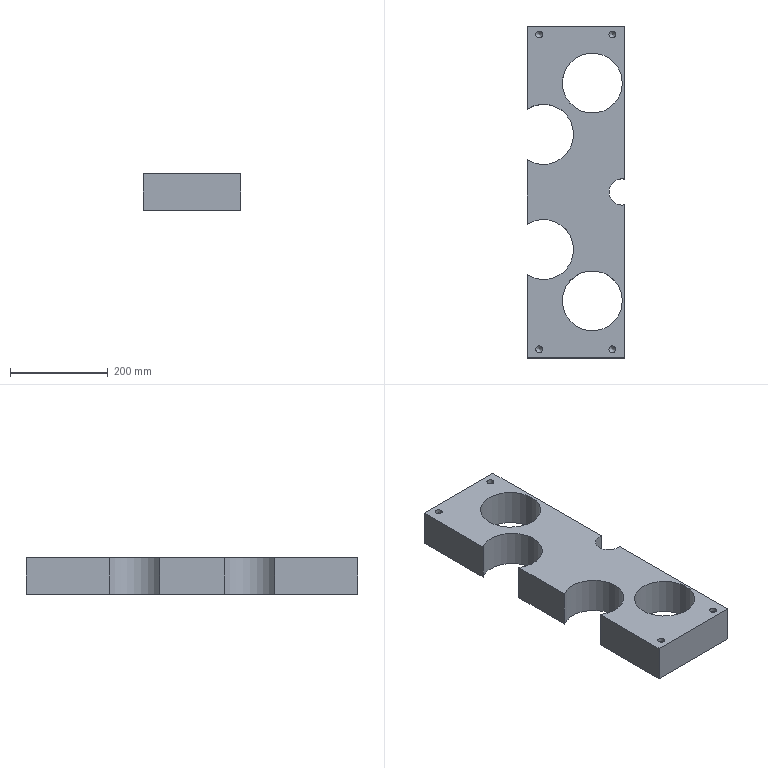Part | NX | features 3 2 | 1 solid | 30 faces | box 199 x 680 x 75.5 mm | volume 6823657 mm3 | cylinder 13 | plane 9 | cone 8 | commonest cylinder face diameters 14.1 x8 123 x4 54 x1
STEP:
#1=CARTESIAN_POINT('',(1737.05,322.5,256.5));
#2=VERTEX_POINT('',#1);
#3=CARTESIAN_POINT('',(1730.,322.5,256.5));
#4=DIRECTION('',(0.,0.,-1.));
#5=DIRECTION('',(1.,0.,0.));
#6=AXIS2_PLACEMENT_3D('',#3,#4,#5);
#7=CIRCLE('',#6,7.05);
#8=EDGE_CURVE('',#2,#2,#7,.T.);
#9=ORIENTED_EDGE('',*,*,#8,.T.);
#10=EDGE_LOOP('',(#9));
#11=FACE_BOUND('',#10,.T.);
#12=CARTESIAN_POINT('',(1587.05,-322.5,256.5));
#13=VERTEX_POINT('',#12);
#14=CARTESIAN_POINT('',(1580.,-322.5,256.5));
#15=DIRECTION('',(0.,0.,-1.));
#16=DIRECTION('',(1.,0.,0.));
#17=AXIS2_PLACEMENT_3D('',#14,#15,#16);
#18=CIRCLE('',#17,7.05);
#19=EDGE_CURVE('',#13,#13,#18,.T.);
#20=ORIENTED_EDGE('',*,*,#19,.T.);
#21=EDGE_LOOP('',(#20));
#22=FACE_BOUND('',#21,.T.);
#23=CARTESIAN_POINT('',(1750.5,-223.,256.5));
#24=VERTEX_POINT('',#23);
#25=CARTESIAN_POINT('',(1689.,-223.,256.5));
#26=DIRECTION('',(0.,0.,1.));
#27=DIRECTION('',(1.,0.,0.));
#28=AXIS2_PLACEMENT_3D('',#25,#26,#27);
#29=CIRCLE('',#28,61.5);
#30=EDGE_CURVE('',#24,#24,#29,.T.);
#31=ORIENTED_EDGE('',*,*,#30,.F.);
#32=EDGE_LOOP('',(#31));
#33=FACE_BOUND('',#32,.T.);
#34=CARTESIAN_POINT('',(1750.5,223.,256.5));
#35=VERTEX_POINT('',#34);
#36=CARTESIAN_POINT('',(1689.,223.,256.5));
#37=DIRECTION('',(0.,0.,-1.));
#38=DIRECTION('',(1.,0.,0.));
#39=AXIS2_PLACEMENT_3D('',#36,#37,#38);
#40=CIRCLE('',#39,61.5);
#41=EDGE_CURVE('',#35,#35,#40,.T.);
#42=ORIENTED_EDGE('',*,*,#41,.T.);
#43=EDGE_LOOP('',(#42));
#44=FACE_BOUND('',#43,.T.);
#45=CARTESIAN_POINT('',(1755.,-26.533,256.5));
#46=VERTEX_POINT('',#45);
#47=CARTESIAN_POINT('',(1755.,-340.,256.5));
#48=VERTEX_POINT('',#47);
#49=CARTESIAN_POINT('',(1755.,193.,256.5));
#50=DIRECTION('',(0.,-1.,0.));
#51=VECTOR('',#50,1000.);
#52=LINE('',#49,#51);
#53=EDGE_CURVE('',#46,#48,#52,.T.);
#54=ORIENTED_EDGE('',*,*,#53,.F.);
#55=CARTESIAN_POINT('',(1755.,26.533,256.5));
#56=VERTEX_POINT('',#55);
#57=CARTESIAN_POINT('',(1750.,0.,256.5));
#58=DIRECTION('',(0.,0.,-1.));
#59=DIRECTION('',(1.,0.,0.));
#60=AXIS2_PLACEMENT_3D('',#57,#58,#59);
#61=CIRCLE('',#60,27.);
#62=EDGE_CURVE('',#46,#56,#61,.T.);
#63=ORIENTED_EDGE('',*,*,#62,.T.);
#64=CARTESIAN_POINT('',(1755.,340.,256.5));
#65=VERTEX_POINT('',#64);
#66=CARTESIAN_POINT('',(1755.,193.,256.5));
#67=DIRECTION('',(0.,-1.,0.));
#68=VECTOR('',#67,1000.);
#69=LINE('',#66,#68);
#70=EDGE_CURVE('',#65,#56,#69,.T.);
#71=ORIENTED_EDGE('',*,*,#70,.F.);
#72=CARTESIAN_POINT('',(1556.,340.,256.5));
#73=VERTEX_POINT('',#72);
#74=CARTESIAN_POINT('',(1447.,340.,256.5));
#75=DIRECTION('',(-1.,0.,0.));
#76=VECTOR('',#75,1000.);
#77=LINE('',#74,#76);
#78=EDGE_CURVE('',#65,#73,#77,.T.);
#79=ORIENTED_EDGE('',*,*,#78,.T.);
#80=CARTESIAN_POINT('',(1556.,169.897,256.5));
#81=VERTEX_POINT('',#80);
#82=CARTESIAN_POINT('',(1556.,-1700.,256.5));
#83=DIRECTION('',(0.,1.,0.));
#84=VECTOR('',#83,1000.);
#85=LINE('',#82,#84);
#86=EDGE_CURVE('',#81,#73,#85,.T.);
#87=ORIENTED_EDGE('',*,*,#86,.F.);
#88=CARTESIAN_POINT('',(1556.,66.103,256.5));
#89=VERTEX_POINT('',#88);
#90=CARTESIAN_POINT('',(1589.,118.,256.5));
#91=DIRECTION('',(0.,0.,1.));
#92=DIRECTION('',(1.,0.,0.));
#93=AXIS2_PLACEMENT_3D('',#90,#91,#92);
#94=CIRCLE('',#93,61.5);
#95=EDGE_CURVE('',#89,#81,#94,.T.);
#96=ORIENTED_EDGE('',*,*,#95,.F.);
#97=CARTESIAN_POINT('',(1556.,-66.103,256.5));
#98=VERTEX_POINT('',#97);
#99=CARTESIAN_POINT('',(1556.,-1700.,256.5));
#100=DIRECTION('',(0.,1.,0.));
#101=VECTOR('',#100,1000.);
#102=LINE('',#99,#101);
#103=EDGE_CURVE('',#98,#89,#102,.T.);
#104=ORIENTED_EDGE('',*,*,#103,.F.);
#105=CARTESIAN_POINT('',(1556.,-169.897,256.5));
#106=VERTEX_POINT('',#105);
#107=CARTESIAN_POINT('',(1589.,-118.,256.5));
#108=DIRECTION('',(0.,0.,-1.));
#109=DIRECTION('',(1.,0.,0.));
#110=AXIS2_PLACEMENT_3D('',#107,#108,#109);
#111=CIRCLE('',#110,61.5);
#112=EDGE_CURVE('',#98,#106,#111,.T.);
#113=ORIENTED_EDGE('',*,*,#112,.T.);
#114=CARTESIAN_POINT('',(1556.,-340.,256.5));
#115=VERTEX_POINT('',#114);
#116=CARTESIAN_POINT('',(1556.,-1700.,256.5));
#117=DIRECTION('',(0.,1.,0.));
#118=VECTOR('',#117,1000.);
#119=LINE('',#116,#118);
#120=EDGE_CURVE('',#115,#106,#119,.T.);
#121=ORIENTED_EDGE('',*,*,#120,.F.);
#122=CARTESIAN_POINT('',(1640.,-340.,256.5));
#123=DIRECTION('',(1.,0.,0.));
#124=VECTOR('',#123,1000.);
#125=LINE('',#122,#124);
#126=EDGE_CURVE('',#115,#48,#125,.T.);
#127=ORIENTED_EDGE('',*,*,#126,.T.);
#128=EDGE_LOOP('',(#54,#63,#71,#79,#87,#96,#104,#113,#121,#127));
#129=FACE_BOUND('',#128,.T.);
#130=CARTESIAN_POINT('',(1587.05,322.5,256.5));
#131=VERTEX_POINT('',#130);
#132=CARTESIAN_POINT('',(1580.,322.5,256.5));
#133=DIRECTION('',(0.,0.,-1.));
#134=DIRECTION('',(1.,0.,0.));
#135=AXIS2_PLACEMENT_3D('',#132,#133,#134);
#136=CIRCLE('',#135,7.05);
#137=EDGE_CURVE('',#131,#131,#136,.T.);
#138=ORIENTED_EDGE('',*,*,#137,.T.);
#139=EDGE_LOOP('',(#138));
#140=FACE_BOUND('',#139,.T.);
#141=CARTESIAN_POINT('',(1737.05,-322.5,256.5));
#142=VERTEX_POINT('',#141);
#143=CARTESIAN_POINT('',(1730.,-322.5,256.5));
#144=DIRECTION('',(0.,0.,-1.));
#145=DIRECTION('',(1.,0.,0.));
#146=AXIS2_PLACEMENT_3D('',#143,#144,#145);
#147=CIRCLE('',#146,7.05);
#148=EDGE_CURVE('',#142,#142,#147,.T.);
#149=ORIENTED_EDGE('',*,*,#148,.T.);
#150=EDGE_LOOP('',(#149));
#151=FACE_BOUND('',#150,.T.);
#152=CARTESIAN_POINT('',(1640.,-1700.,256.5));
#153=DIRECTION('',(0.,0.,1.));
#154=DIRECTION('',(0.,1.,0.));
#155=AXIS2_PLACEMENT_3D('',#152,#153,#154);
#156=PLANE('',#155);
#157=ADVANCED_FACE('',(#11,#22,#33,#44,#129,#140,#151),#156,.T.);
#158=CARTESIAN_POINT('',(1738.05,-127.5,181.));
#159=VERTEX_POINT('',#158);
#160=CARTESIAN_POINT('',(1731.,-127.5,181.));
#161=DIRECTION('',(0.,0.,1.));
#162=DIRECTION('',(1.,0.,0.));
#163=AXIS2_PLACEMENT_3D('',#160,#161,#162);
#164=CIRCLE('',#163,7.05);
#165=EDGE_CURVE('',#159,#159,#164,.T.);
#166=ORIENTED_EDGE('',*,*,#165,.T.);
#167=EDGE_LOOP('',(#166));
#168=FACE_BOUND('',#167,.T.);
#169=CARTESIAN_POINT('',(1738.05,127.5,181.));
#170=VERTEX_POINT('',#169);
#171=CARTESIAN_POINT('',(1731.,127.5,181.));
#172=DIRECTION('',(0.,0.,1.));
#173=DIRECTION('',(1.,0.,0.));
#174=AXIS2_PLACEMENT_3D('',#171,#172,#173);
#175=CIRCLE('',#174,7.05);
#176=EDGE_CURVE('',#170,#170,#175,.T.);
#177=ORIENTED_EDGE('',*,*,#176,.T.);
#178=EDGE_LOOP('',(#177));
#179=FACE_BOUND('',#178,.T.);
#180=CARTESIAN_POINT('',(1627.5,-223.,181.));
#181=VERTEX_POINT('',#180);
#182=CARTESIAN_POINT('',(1689.,-223.,181.));
#183=DIRECTION('',(0.,0.,-1.));
#184=DIRECTION('',(-1.,0.,0.));
#185=AXIS2_PLACEMENT_3D('',#182,#183,#184);
#186=CIRCLE('',#185,61.5);
#187=EDGE_CURVE('',#181,#181,#186,.T.);
#188=ORIENTED_EDGE('',*,*,#187,.F.);
#189=EDGE_LOOP('',(#188));
#190=FACE_BOUND('',#189,.T.);
#191=CARTESIAN_POINT('',(1627.5,223.,181.));
#192=VERTEX_POINT('',#191);
#193=CARTESIAN_POINT('',(1689.,223.,181.));
#194=DIRECTION('',(0.,0.,1.));
#195=DIRECTION('',(-1.,0.,0.));
#196=AXIS2_PLACEMENT_3D('',#193,#194,#195);
#197=CIRCLE('',#196,61.5);
#198=EDGE_CURVE('',#192,#192,#197,.T.);
#199=ORIENTED_EDGE('',*,*,#198,.T.);
#200=EDGE_LOOP('',(#199));
#201=FACE_BOUND('',#200,.T.);
#202=CARTESIAN_POINT('',(1755.,26.533,181.));
#203=VERTEX_POINT('',#202);
#204=CARTESIAN_POINT('',(1755.,340.,181.));
#205=VERTEX_POINT('',#204);
#206=CARTESIAN_POINT('',(1755.,193.,181.));
#207=DIRECTION('',(0.,1.,0.));
#208=VECTOR('',#207,1000.);
#209=LINE('',#206,#208);
#210=EDGE_CURVE('',#203,#205,#209,.T.);
#211=ORIENTED_EDGE('',*,*,#210,.F.);
#212=CARTESIAN_POINT('',(1755.,-26.533,181.));
#213=VERTEX_POINT('',#212);
#214=CARTESIAN_POINT('',(1750.,0.,181.));
#215=DIRECTION('',(0.,0.,1.));
#216=DIRECTION('',(-1.,0.,0.));
#217=AXIS2_PLACEMENT_3D('',#214,#215,#216);
#218=CIRCLE('',#217,27.);
#219=EDGE_CURVE('',#203,#213,#218,.T.);
#220=ORIENTED_EDGE('',*,*,#219,.T.);
#221=CARTESIAN_POINT('',(1755.,-340.,181.));
#222=VERTEX_POINT('',#221);
#223=CARTESIAN_POINT('',(1755.,193.,181.));
#224=DIRECTION('',(0.,1.,0.));
#225=VECTOR('',#224,1000.);
#226=LINE('',#223,#225);
#227=EDGE_CURVE('',#222,#213,#226,.T.);
#228=ORIENTED_EDGE('',*,*,#227,.F.);
#229=CARTESIAN_POINT('',(1556.,-340.,181.));
#230=VERTEX_POINT('',#229);
#231=CARTESIAN_POINT('',(1447.,-340.,181.));
#232=DIRECTION('',(-1.,0.,0.));
#233=VECTOR('',#232,1000.);
#234=LINE('',#231,#233);
#235=EDGE_CURVE('',#222,#230,#234,.T.);
#236=ORIENTED_EDGE('',*,*,#235,.T.);
#237=CARTESIAN_POINT('',(1556.,-169.897,181.));
#238=VERTEX_POINT('',#237);
#239=CARTESIAN_POINT('',(1556.,-930.,181.));
#240=DIRECTION('',(0.,-1.,0.));
#241=VECTOR('',#240,1000.);
#242=LINE('',#239,#241);
#243=EDGE_CURVE('',#238,#230,#242,.T.);
#244=ORIENTED_EDGE('',*,*,#243,.F.);
#245=CARTESIAN_POINT('',(1556.,-66.103,181.));
#246=VERTEX_POINT('',#245);
#247=CARTESIAN_POINT('',(1589.,-118.,181.));
#248=DIRECTION('',(0.,0.,-1.));
#249=DIRECTION('',(-1.,0.,0.));
#250=AXIS2_PLACEMENT_3D('',#247,#248,#249);
#251=CIRCLE('',#250,61.5);
#252=EDGE_CURVE('',#246,#238,#251,.T.);
#253=ORIENTED_EDGE('',*,*,#252,.F.);
#254=CARTESIAN_POINT('',(1556.,66.103,181.));
#255=VERTEX_POINT('',#254);
#256=CARTESIAN_POINT('',(1556.,-930.,181.));
#257=DIRECTION('',(0.,-1.,0.));
#258=VECTOR('',#257,1000.);
#259=LINE('',#256,#258);
#260=EDGE_CURVE('',#255,#246,#259,.T.);
#261=ORIENTED_EDGE('',*,*,#260,.F.);
#262=CARTESIAN_POINT('',(1556.,169.897,181.));
#263=VERTEX_POINT('',#262);
#264=CARTESIAN_POINT('',(1589.,118.,181.));
#265=DIRECTION('',(0.,0.,1.));
#266=DIRECTION('',(-1.,0.,0.));
#267=AXIS2_PLACEMENT_3D('',#264,#265,#266);
#268=CIRCLE('',#267,61.5);
#269=EDGE_CURVE('',#255,#263,#268,.T.);
#270=ORIENTED_EDGE('',*,*,#269,.T.);
#271=CARTESIAN_POINT('',(1556.,340.,181.));
#272=VERTEX_POINT('',#271);
#273=CARTESIAN_POINT('',(1556.,-930.,181.));
#274=DIRECTION('',(0.,-1.,0.));
#275=VECTOR('',#274,1000.);
#276=LINE('',#273,#275);
#277=EDGE_CURVE('',#272,#263,#276,.T.);
#278=ORIENTED_EDGE('',*,*,#277,.F.);
#279=CARTESIAN_POINT('',(1447.,340.,181.));
#280=DIRECTION('',(1.,0.,0.));
#281=VECTOR('',#280,1000.);
#282=LINE('',#279,#281);
#283=EDGE_CURVE('',#272,#205,#282,.T.);
#284=ORIENTED_EDGE('',*,*,#283,.T.);
#285=EDGE_LOOP('',(#211,#220,#228,#236,#244,#253,#261,#270,#278,#284));
#286=FACE_BOUND('',#285,.T.);
#287=CARTESIAN_POINT('',(1587.05,-322.5,181.));
#288=VERTEX_POINT('',#287);
#289=CARTESIAN_POINT('',(1580.,-322.5,181.));
#290=DIRECTION('',(0.,0.,1.));
#291=DIRECTION('',(1.,0.,0.));
#292=AXIS2_PLACEMENT_3D('',#289,#290,#291);
#293=CIRCLE('',#292,7.05);
#294=EDGE_CURVE('',#288,#288,#293,.T.);
#295=ORIENTED_EDGE('',*,*,#294,.T.);
#296=EDGE_LOOP('',(#295));
#297=FACE_BOUND('',#296,.T.);
#298=CARTESIAN_POINT('',(1587.05,322.5,181.));
#299=VERTEX_POINT('',#298);
#300=CARTESIAN_POINT('',(1580.,322.5,181.));
#301=DIRECTION('',(0.,0.,1.));
#302=DIRECTION('',(1.,0.,0.));
#303=AXIS2_PLACEMENT_3D('',#300,#301,#302);
#304=CIRCLE('',#303,7.05);
#305=EDGE_CURVE('',#299,#299,#304,.T.);
#306=ORIENTED_EDGE('',*,*,#305,.T.);
#307=EDGE_LOOP('',(#306));
#308=FACE_BOUND('',#307,.T.);
#309=CARTESIAN_POINT('',(1447.,-930.,181.));
#310=DIRECTION('',(0.,0.,-1.));
#311=DIRECTION('',(0.,1.,0.));
#312=AXIS2_PLACEMENT_3D('',#309,#310,#311);
#313=PLANE('',#312);
#314=ADVANCED_FACE('',(#168,#179,#190,#201,#286,#297,#308),#313,.T.);
#315=ORIENTED_EDGE('',*,*,#70,.T.);
#316=CARTESIAN_POINT('',(1755.,26.533,-181.));
#317=DIRECTION('',(0.,0.,-1.));
#318=VECTOR('',#317,1000.);
#319=LINE('',#316,#318);
#320=EDGE_CURVE('',#56,#203,#319,.T.);
#321=ORIENTED_EDGE('',*,*,#320,.T.);
#322=ORIENTED_EDGE('',*,*,#210,.T.);
#323=CARTESIAN_POINT('',(1755.,340.,-1.5));
#324=DIRECTION('',(0.,0.,1.));
#325=VECTOR('',#324,1000.);
#326=LINE('',#323,#325);
#327=EDGE_CURVE('',#205,#65,#326,.T.);
#328=ORIENTED_EDGE('',*,*,#327,.T.);
#329=EDGE_LOOP('',(#315,#321,#322,#328));
#330=FACE_BOUND('',#329,.T.);
#331=CARTESIAN_POINT('',(1755.,193.,-1.5));
#332=DIRECTION('',(1.,0.,0.));
#333=DIRECTION('',(0.,0.,1.));
#334=AXIS2_PLACEMENT_3D('',#331,#332,#333);
#335=PLANE('',#334);
#336=ADVANCED_FACE('',(#330),#335,.T.);
#337=ORIENTED_EDGE('',*,*,#227,.T.);
#338=CARTESIAN_POINT('',(1755.,-26.533,-181.));
#339=DIRECTION('',(0.,0.,1.));
#340=VECTOR('',#339,1000.);
#341=LINE('',#338,#340);
#342=EDGE_CURVE('',#213,#46,#341,.T.);
#343=ORIENTED_EDGE('',*,*,#342,.T.);
#344=ORIENTED_EDGE('',*,*,#53,.T.);
#345=CARTESIAN_POINT('',(1755.,-340.,-1.5));
#346=DIRECTION('',(0.,0.,-1.));
#347=VECTOR('',#346,1000.);
#348=LINE('',#345,#347);
#349=EDGE_CURVE('',#48,#222,#348,.T.);
#350=ORIENTED_EDGE('',*,*,#349,.T.);
#351=EDGE_LOOP('',(#337,#343,#344,#350));
#352=FACE_BOUND('',#351,.T.);
#353=CARTESIAN_POINT('',(1755.,193.,-1.5));
#354=DIRECTION('',(1.,0.,0.));
#355=DIRECTION('',(0.,0.,1.));
#356=AXIS2_PLACEMENT_3D('',#353,#354,#355);
#357=PLANE('',#356);
#358=ADVANCED_FACE('',(#352),#357,.T.);
#359=ORIENTED_EDGE('',*,*,#103,.T.);
#360=CARTESIAN_POINT('',(1556.,66.103,-181.));
#361=DIRECTION('',(0.,0.,-1.));
#362=VECTOR('',#361,1000.);
#363=LINE('',#360,#362);
#364=EDGE_CURVE('',#89,#255,#363,.T.);
#365=ORIENTED_EDGE('',*,*,#364,.T.);
#366=ORIENTED_EDGE('',*,*,#260,.T.);
#367=CARTESIAN_POINT('',(1556.,-66.103,-181.));
#368=DIRECTION('',(0.,0.,1.));
#369=VECTOR('',#368,1000.);
#370=LINE('',#367,#369);
#371=EDGE_CURVE('',#246,#98,#370,.T.);
#372=ORIENTED_EDGE('',*,*,#371,.T.);
#373=EDGE_LOOP('',(#359,#365,#366,#372));
#374=FACE_BOUND('',#373,.T.);
#375=CARTESIAN_POINT('',(1556.,315.,218.75));
#376=DIRECTION('',(-1.,0.,0.));
#377=DIRECTION('',(0.,0.,-1.));
#378=AXIS2_PLACEMENT_3D('',#375,#376,#377);
#379=PLANE('',#378);
#380=ADVANCED_FACE('',(#374),#379,.T.);
#381=ORIENTED_EDGE('',*,*,#277,.T.);
#382=CARTESIAN_POINT('',(1556.,169.897,-181.));
#383=DIRECTION('',(0.,0.,1.));
#384=VECTOR('',#383,1000.);
#385=LINE('',#382,#384);
#386=EDGE_CURVE('',#263,#81,#385,.T.);
#387=ORIENTED_EDGE('',*,*,#386,.T.);
#388=ORIENTED_EDGE('',*,*,#86,.T.);
#389=CARTESIAN_POINT('',(1556.,340.,-1.5));
#390=DIRECTION('',(0.,0.,-1.));
#391=VECTOR('',#390,1000.);
#392=LINE('',#389,#391);
#393=EDGE_CURVE('',#73,#272,#392,.T.);
#394=ORIENTED_EDGE('',*,*,#393,.T.);
#395=EDGE_LOOP('',(#381,#387,#388,#394));
#396=FACE_BOUND('',#395,.T.);
#397=CARTESIAN_POINT('',(1556.,315.,218.75));
#398=DIRECTION('',(-1.,0.,0.));
#399=DIRECTION('',(0.,0.,-1.));
#400=AXIS2_PLACEMENT_3D('',#397,#398,#399);
#401=PLANE('',#400);
#402=ADVANCED_FACE('',(#396),#401,.T.);
#403=ORIENTED_EDGE('',*,*,#120,.T.);
#404=CARTESIAN_POINT('',(1556.,-169.897,-181.));
#405=DIRECTION('',(0.,0.,-1.));
#406=VECTOR('',#405,1000.);
#407=LINE('',#404,#406);
#408=EDGE_CURVE('',#106,#238,#407,.T.);
#409=ORIENTED_EDGE('',*,*,#408,.T.);
#410=ORIENTED_EDGE('',*,*,#243,.T.);
#411=CARTESIAN_POINT('',(1556.,-340.,218.75));
#412=DIRECTION('',(0.,0.,1.));
#413=VECTOR('',#412,1000.);
#414=LINE('',#411,#413);
#415=EDGE_CURVE('',#230,#115,#414,.T.);
#416=ORIENTED_EDGE('',*,*,#415,.T.);
#417=EDGE_LOOP('',(#403,#409,#410,#416));
#418=FACE_BOUND('',#417,.T.);
#419=CARTESIAN_POINT('',(1556.,315.,218.75));
#420=DIRECTION('',(-1.,0.,0.));
#421=DIRECTION('',(0.,0.,-1.));
#422=AXIS2_PLACEMENT_3D('',#419,#420,#421);
#423=PLANE('',#422);
#424=ADVANCED_FACE('',(#418),#423,.T.);
#425=ORIENTED_EDGE('',*,*,#283,.F.);
#426=ORIENTED_EDGE('',*,*,#393,.F.);
#427=ORIENTED_EDGE('',*,*,#78,.F.);
#428=ORIENTED_EDGE('',*,*,#327,.F.);
#429=EDGE_LOOP('',(#425,#426,#427,#428));
#430=FACE_BOUND('',#429,.T.);
#431=CARTESIAN_POINT('',(1447.,340.,-1.5));
#432=DIRECTION('',(0.,1.,0.));
#433=DIRECTION('',(0.,0.,-1.));
#434=AXIS2_PLACEMENT_3D('',#431,#432,#433);
#435=PLANE('',#434);
#436=ADVANCED_FACE('',(#430),#435,.T.);
#437=ORIENTED_EDGE('',*,*,#126,.F.);
#438=ORIENTED_EDGE('',*,*,#415,.F.);
#439=ORIENTED_EDGE('',*,*,#235,.F.);
#440=ORIENTED_EDGE('',*,*,#349,.F.);
#441=EDGE_LOOP('',(#437,#438,#439,#440));
#442=FACE_BOUND('',#441,.T.);
#443=CARTESIAN_POINT('',(1447.,-340.,-1.5));
#444=DIRECTION('',(0.,-1.,0.));
#445=DIRECTION('',(0.,0.,-1.));
#446=AXIS2_PLACEMENT_3D('',#443,#444,#445);
#447=PLANE('',#446);
#448=ADVANCED_FACE('',(#442),#447,.T.);
#449=ORIENTED_EDGE('',*,*,#30,.T.);
#450=EDGE_LOOP('',(#449));
#451=FACE_BOUND('',#450,.T.);
#452=ORIENTED_EDGE('',*,*,#187,.T.);
#453=EDGE_LOOP('',(#452));
#454=FACE_BOUND('',#453,.T.);
#455=CARTESIAN_POINT('',(1689.,-223.,-181.));
#456=DIRECTION('',(0.,0.,1.));
#457=DIRECTION('',(-1.,0.,0.));
#458=AXIS2_PLACEMENT_3D('',#455,#456,#457);
#459=CYLINDRICAL_SURFACE('',#458,61.5);
#460=ADVANCED_FACE('',(#451,#454),#459,.F.);
#461=ORIENTED_EDGE('',*,*,#408,.F.);
#462=ORIENTED_EDGE('',*,*,#112,.F.);
#463=ORIENTED_EDGE('',*,*,#371,.F.);
#464=ORIENTED_EDGE('',*,*,#252,.T.);
#465=EDGE_LOOP('',(#461,#462,#463,#464));
#466=FACE_BOUND('',#465,.T.);
#467=CARTESIAN_POINT('',(1589.,-118.,-181.));
#468=DIRECTION('',(0.,0.,1.));
#469=DIRECTION('',(-1.,0.,0.));
#470=AXIS2_PLACEMENT_3D('',#467,#468,#469);
#471=CYLINDRICAL_SURFACE('',#470,61.5);
#472=ADVANCED_FACE('',(#466),#471,.F.);
#473=ORIENTED_EDGE('',*,*,#364,.F.);
#474=ORIENTED_EDGE('',*,*,#95,.T.);
#475=ORIENTED_EDGE('',*,*,#386,.F.);
#476=ORIENTED_EDGE('',*,*,#269,.F.);
#477=EDGE_LOOP('',(#473,#474,#475,#476));
#478=FACE_BOUND('',#477,.T.);
#479=CARTESIAN_POINT('',(1589.,118.,-181.));
#480=DIRECTION('',(0.,0.,1.));
#481=DIRECTION('',(-1.,0.,0.));
#482=AXIS2_PLACEMENT_3D('',#479,#480,#481);
#483=CYLINDRICAL_SURFACE('',#482,61.5);
#484=ADVANCED_FACE('',(#478),#483,.F.);
#485=ORIENTED_EDGE('',*,*,#41,.F.);
#486=EDGE_LOOP('',(#485));
#487=FACE_BOUND('',#486,.T.);
#488=ORIENTED_EDGE('',*,*,#198,.F.);
#489=EDGE_LOOP('',(#488));
#490=FACE_BOUND('',#489,.T.);
#491=CARTESIAN_POINT('',(1689.,223.,-181.));
#492=DIRECTION('',(0.,0.,1.));
#493=DIRECTION('',(-1.,0.,0.));
#494=AXIS2_PLACEMENT_3D('',#491,#492,#493);
#495=CYLINDRICAL_SURFACE('',#494,61.5);
#496=ADVANCED_FACE('',(#487,#490),#495,.F.);
#497=ORIENTED_EDGE('',*,*,#320,.F.);
#498=ORIENTED_EDGE('',*,*,#62,.F.);
#499=ORIENTED_EDGE('',*,*,#342,.F.);
#500=ORIENTED_EDGE('',*,*,#219,.F.);
#501=EDGE_LOOP('',(#497,#498,#499,#500));
#502=FACE_BOUND('',#501,.T.);
#503=CARTESIAN_POINT('',(1750.,0.,-181.));
#504=DIRECTION('',(0.,0.,1.));
#505=DIRECTION('',(-1.,0.,0.));
#506=AXIS2_PLACEMENT_3D('',#503,#504,#505);
#507=CYLINDRICAL_SURFACE('',#506,27.);
#508=ADVANCED_FACE('',(#502),#507,.F.);
#509=CARTESIAN_POINT('',(1738.05,127.5,188.95));
#510=VERTEX_POINT('',#509);
#511=CARTESIAN_POINT('',(1731.,127.5,188.95));
#512=DIRECTION('',(0.,0.,1.));
#513=DIRECTION('',(1.,0.,0.));
#514=AXIS2_PLACEMENT_3D('',#511,#512,#513);
#515=CIRCLE('',#514,7.05);
#516=EDGE_CURVE('',#510,#510,#515,.T.);
#517=ORIENTED_EDGE('',*,*,#516,.T.);
#518=EDGE_LOOP('',(#517));
#519=FACE_BOUND('',#518,.T.);
#520=ORIENTED_EDGE('',*,*,#176,.F.);
#521=EDGE_LOOP('',(#520));
#522=FACE_BOUND('',#521,.T.);
#523=CARTESIAN_POINT('',(1731.,127.5,181.));
#524=DIRECTION('',(0.,0.,1.));
#525=DIRECTION('',(-1.,0.,0.));
#526=AXIS2_PLACEMENT_3D('',#523,#524,#525);
#527=CYLINDRICAL_SURFACE('',#526,7.05);
#528=ADVANCED_FACE('',(#519,#522),#527,.F.);
#529=CARTESIAN_POINT('',(1731.,127.5,196.));
#530=VERTEX_POINT('',#529);
#531=VERTEX_LOOP('',#530);
#532=FACE_BOUND('',#531,.T.);
#533=ORIENTED_EDGE('',*,*,#516,.F.);
#534=EDGE_LOOP('',(#533));
#535=FACE_BOUND('',#534,.T.);
#536=CARTESIAN_POINT('',(1731.,127.5,188.95));
#537=DIRECTION('',(0.,0.,-1.));
#538=DIRECTION('',(1.,0.,0.));
#539=AXIS2_PLACEMENT_3D('',#536,#537,#538);
#540=CONICAL_SURFACE('',#539,7.05,0.7854);
#541=ADVANCED_FACE('',(#532,#535),#540,.F.);
#542=CARTESIAN_POINT('',(1587.05,-322.5,188.95));
#543=VERTEX_POINT('',#542);
#544=CARTESIAN_POINT('',(1580.,-322.5,188.95));
#545=DIRECTION('',(0.,0.,1.));
#546=DIRECTION('',(1.,0.,0.));
#547=AXIS2_PLACEMENT_3D('',#544,#545,#546);
#548=CIRCLE('',#547,7.05);
#549=EDGE_CURVE('',#543,#543,#548,.T.);
#550=ORIENTED_EDGE('',*,*,#549,.T.);
#551=EDGE_LOOP('',(#550));
#552=FACE_BOUND('',#551,.T.);
#553=ORIENTED_EDGE('',*,*,#294,.F.);
#554=EDGE_LOOP('',(#553));
#555=FACE_BOUND('',#554,.T.);
#556=CARTESIAN_POINT('',(1580.,-322.5,181.));
#557=DIRECTION('',(0.,0.,1.));
#558=DIRECTION('',(-1.,0.,0.));
#559=AXIS2_PLACEMENT_3D('',#556,#557,#558);
#560=CYLINDRICAL_SURFACE('',#559,7.05);
#561=ADVANCED_FACE('',(#552,#555),#560,.F.);
#562=CARTESIAN_POINT('',(1580.,-322.5,196.));
#563=VERTEX_POINT('',#562);
#564=VERTEX_LOOP('',#563);
#565=FACE_BOUND('',#564,.T.);
#566=ORIENTED_EDGE('',*,*,#549,.F.);
#567=EDGE_LOOP('',(#566));
#568=FACE_BOUND('',#567,.T.);
#569=CARTESIAN_POINT('',(1580.,-322.5,188.95));
#570=DIRECTION('',(0.,0.,-1.));
#571=DIRECTION('',(1.,0.,0.));
#572=AXIS2_PLACEMENT_3D('',#569,#570,#571);
#573=CONICAL_SURFACE('',#572,7.05,0.7854);
#574=ADVANCED_FACE('',(#565,#568),#573,.F.);
#575=CARTESIAN_POINT('',(1738.05,-127.5,188.95));
#576=VERTEX_POINT('',#575);
#577=CARTESIAN_POINT('',(1731.,-127.5,188.95));
#578=DIRECTION('',(0.,0.,1.));
#579=DIRECTION('',(1.,0.,0.));
#580=AXIS2_PLACEMENT_3D('',#577,#578,#579);
#581=CIRCLE('',#580,7.05);
#582=EDGE_CURVE('',#576,#576,#581,.T.);
#583=ORIENTED_EDGE('',*,*,#582,.T.);
#584=EDGE_LOOP('',(#583));
#585=FACE_BOUND('',#584,.T.);
#586=ORIENTED_EDGE('',*,*,#165,.F.);
#587=EDGE_LOOP('',(#586));
#588=FACE_BOUND('',#587,.T.);
#589=CARTESIAN_POINT('',(1731.,-127.5,181.));
#590=DIRECTION('',(0.,0.,1.));
#591=DIRECTION('',(-1.,0.,0.));
#592=AXIS2_PLACEMENT_3D('',#589,#590,#591);
#593=CYLINDRICAL_SURFACE('',#592,7.05);
#594=ADVANCED_FACE('',(#585,#588),#593,.F.);
#595=CARTESIAN_POINT('',(1731.,-127.5,196.));
#596=VERTEX_POINT('',#595);
#597=VERTEX_LOOP('',#596);
#598=FACE_BOUND('',#597,.T.);
#599=ORIENTED_EDGE('',*,*,#582,.F.);
#600=EDGE_LOOP('',(#599));
#601=FACE_BOUND('',#600,.T.);
#602=CARTESIAN_POINT('',(1731.,-127.5,188.95));
#603=DIRECTION('',(0.,0.,-1.));
#604=DIRECTION('',(1.,0.,0.));
#605=AXIS2_PLACEMENT_3D('',#602,#603,#604);
#606=CONICAL_SURFACE('',#605,7.05,0.7854);
#607=ADVANCED_FACE('',(#598,#601),#606,.F.);
#608=CARTESIAN_POINT('',(1587.05,322.5,188.95));
#609=VERTEX_POINT('',#608);
#610=CARTESIAN_POINT('',(1580.,322.5,188.95));
#611=DIRECTION('',(0.,0.,1.));
#612=DIRECTION('',(1.,0.,0.));
#613=AXIS2_PLACEMENT_3D('',#610,#611,#612);
#614=CIRCLE('',#613,7.05);
#615=EDGE_CURVE('',#609,#609,#614,.T.);
#616=ORIENTED_EDGE('',*,*,#615,.T.);
#617=EDGE_LOOP('',(#616));
#618=FACE_BOUND('',#617,.T.);
#619=ORIENTED_EDGE('',*,*,#305,.F.);
#620=EDGE_LOOP('',(#619));
#621=FACE_BOUND('',#620,.T.);
#622=CARTESIAN_POINT('',(1580.,322.5,181.));
#623=DIRECTION('',(0.,0.,1.));
#624=DIRECTION('',(-1.,0.,0.));
#625=AXIS2_PLACEMENT_3D('',#622,#623,#624);
#626=CYLINDRICAL_SURFACE('',#625,7.05);
#627=ADVANCED_FACE('',(#618,#621),#626,.F.);
#628=CARTESIAN_POINT('',(1580.,322.5,196.));
#629=VERTEX_POINT('',#628);
#630=VERTEX_LOOP('',#629);
#631=FACE_BOUND('',#630,.T.);
#632=ORIENTED_EDGE('',*,*,#615,.F.);
#633=EDGE_LOOP('',(#632));
#634=FACE_BOUND('',#633,.T.);
#635=CARTESIAN_POINT('',(1580.,322.5,188.95));
#636=DIRECTION('',(0.,0.,-1.));
#637=DIRECTION('',(1.,0.,0.));
#638=AXIS2_PLACEMENT_3D('',#635,#636,#637);
#639=CONICAL_SURFACE('',#638,7.05,0.7854);
#640=ADVANCED_FACE('',(#631,#634),#639,.F.);
#641=CARTESIAN_POINT('',(1572.95,-322.5,248.55));
#642=VERTEX_POINT('',#641);
#643=CARTESIAN_POINT('',(1580.,-322.5,248.55));
#644=DIRECTION('',(0.,0.,-1.));
#645=DIRECTION('',(-1.,0.,0.));
#646=AXIS2_PLACEMENT_3D('',#643,#644,#645);
#647=CIRCLE('',#646,7.05);
#648=EDGE_CURVE('',#642,#642,#647,.T.);
#649=ORIENTED_EDGE('',*,*,#648,.T.);
#650=EDGE_LOOP('',(#649));
#651=FACE_BOUND('',#650,.T.);
#652=ORIENTED_EDGE('',*,*,#19,.F.);
#653=EDGE_LOOP('',(#652));
#654=FACE_BOUND('',#653,.T.);
#655=CARTESIAN_POINT('',(1580.,-322.5,256.5));
#656=DIRECTION('',(0.,0.,-1.));
#657=DIRECTION('',(-1.,0.,0.));
#658=AXIS2_PLACEMENT_3D('',#655,#656,#657);
#659=CYLINDRICAL_SURFACE('',#658,7.05);
#660=ADVANCED_FACE('',(#651,#654),#659,.F.);
#661=CARTESIAN_POINT('',(1580.,-322.5,241.5));
#662=VERTEX_POINT('',#661);
#663=VERTEX_LOOP('',#662);
#664=FACE_BOUND('',#663,.T.);
#665=ORIENTED_EDGE('',*,*,#648,.F.);
#666=EDGE_LOOP('',(#665));
#667=FACE_BOUND('',#666,.T.);
#668=CARTESIAN_POINT('',(1580.,-322.5,248.55));
#669=DIRECTION('',(0.,0.,1.));
#670=DIRECTION('',(-1.,0.,0.));
#671=AXIS2_PLACEMENT_3D('',#668,#669,#670);
#672=CONICAL_SURFACE('',#671,7.05,0.7854);
#673=ADVANCED_FACE('',(#664,#667),#672,.F.);
#674=CARTESIAN_POINT('',(1572.95,322.5,248.55));
#675=VERTEX_POINT('',#674);
#676=CARTESIAN_POINT('',(1580.,322.5,248.55));
#677=DIRECTION('',(0.,0.,-1.));
#678=DIRECTION('',(-1.,0.,0.));
#679=AXIS2_PLACEMENT_3D('',#676,#677,#678);
#680=CIRCLE('',#679,7.05);
#681=EDGE_CURVE('',#675,#675,#680,.T.);
#682=ORIENTED_EDGE('',*,*,#681,.T.);
#683=EDGE_LOOP('',(#682));
#684=FACE_BOUND('',#683,.T.);
#685=ORIENTED_EDGE('',*,*,#137,.F.);
#686=EDGE_LOOP('',(#685));
#687=FACE_BOUND('',#686,.T.);
#688=CARTESIAN_POINT('',(1580.,322.5,256.5));
#689=DIRECTION('',(0.,0.,-1.));
#690=DIRECTION('',(-1.,0.,0.));
#691=AXIS2_PLACEMENT_3D('',#688,#689,#690);
#692=CYLINDRICAL_SURFACE('',#691,7.05);
#693=ADVANCED_FACE('',(#684,#687),#692,.F.);
#694=CARTESIAN_POINT('',(1580.,322.5,241.5));
#695=VERTEX_POINT('',#694);
#696=VERTEX_LOOP('',#695);
#697=FACE_BOUND('',#696,.T.);
#698=ORIENTED_EDGE('',*,*,#681,.F.);
#699=EDGE_LOOP('',(#698));
#700=FACE_BOUND('',#699,.T.);
#701=CARTESIAN_POINT('',(1580.,322.5,248.55));
#702=DIRECTION('',(0.,0.,1.));
#703=DIRECTION('',(-1.,0.,0.));
#704=AXIS2_PLACEMENT_3D('',#701,#702,#703);
#705=CONICAL_SURFACE('',#704,7.05,0.7854);
#706=ADVANCED_FACE('',(#697,#700),#705,.F.);
#707=CARTESIAN_POINT('',(1722.95,322.5,248.55));
#708=VERTEX_POINT('',#707);
#709=CARTESIAN_POINT('',(1730.,322.5,248.55));
#710=DIRECTION('',(0.,0.,-1.));
#711=DIRECTION('',(-1.,0.,0.));
#712=AXIS2_PLACEMENT_3D('',#709,#710,#711);
#713=CIRCLE('',#712,7.05);
#714=EDGE_CURVE('',#708,#708,#713,.T.);
#715=ORIENTED_EDGE('',*,*,#714,.T.);
#716=EDGE_LOOP('',(#715));
#717=FACE_BOUND('',#716,.T.);
#718=ORIENTED_EDGE('',*,*,#8,.F.);
#719=EDGE_LOOP('',(#718));
#720=FACE_BOUND('',#719,.T.);
#721=CARTESIAN_POINT('',(1730.,322.5,256.5));
#722=DIRECTION('',(0.,0.,-1.));
#723=DIRECTION('',(-1.,0.,0.));
#724=AXIS2_PLACEMENT_3D('',#721,#722,#723);
#725=CYLINDRICAL_SURFACE('',#724,7.05);
#726=ADVANCED_FACE('',(#717,#720),#725,.F.);
#727=CARTESIAN_POINT('',(1730.,322.5,241.5));
#728=VERTEX_POINT('',#727);
#729=VERTEX_LOOP('',#728);
#730=FACE_BOUND('',#729,.T.);
#731=ORIENTED_EDGE('',*,*,#714,.F.);
#732=EDGE_LOOP('',(#731));
#733=FACE_BOUND('',#732,.T.);
#734=CARTESIAN_POINT('',(1730.,322.5,248.55));
#735=DIRECTION('',(0.,0.,1.));
#736=DIRECTION('',(-1.,0.,0.));
#737=AXIS2_PLACEMENT_3D('',#734,#735,#736);
#738=CONICAL_SURFACE('',#737,7.05,0.7854);
#739=ADVANCED_FACE('',(#730,#733),#738,.F.);
#740=CARTESIAN_POINT('',(1722.95,-322.5,248.55));
#741=VERTEX_POINT('',#740);
#742=CARTESIAN_POINT('',(1730.,-322.5,248.55));
#743=DIRECTION('',(0.,0.,-1.));
#744=DIRECTION('',(-1.,0.,0.));
#745=AXIS2_PLACEMENT_3D('',#742,#743,#744);
#746=CIRCLE('',#745,7.05);
#747=EDGE_CURVE('',#741,#741,#746,.T.);
#748=ORIENTED_EDGE('',*,*,#747,.T.);
#749=EDGE_LOOP('',(#748));
#750=FACE_BOUND('',#749,.T.);
#751=ORIENTED_EDGE('',*,*,#148,.F.);
#752=EDGE_LOOP('',(#751));
#753=FACE_BOUND('',#752,.T.);
#754=CARTESIAN_POINT('',(1730.,-322.5,256.5));
#755=DIRECTION('',(0.,0.,-1.));
#756=DIRECTION('',(-1.,0.,0.));
#757=AXIS2_PLACEMENT_3D('',#754,#755,#756);
#758=CYLINDRICAL_SURFACE('',#757,7.05);
#759=ADVANCED_FACE('',(#750,#753),#758,.F.);
#760=CARTESIAN_POINT('',(1730.,-322.5,241.5));
#761=VERTEX_POINT('',#760);
#762=VERTEX_LOOP('',#761);
#763=FACE_BOUND('',#762,.T.);
#764=ORIENTED_EDGE('',*,*,#747,.F.);
#765=EDGE_LOOP('',(#764));
#766=FACE_BOUND('',#765,.T.);
#767=CARTESIAN_POINT('',(1730.,-322.5,248.55));
#768=DIRECTION('',(0.,0.,1.));
#769=DIRECTION('',(-1.,0.,0.));
#770=AXIS2_PLACEMENT_3D('',#767,#768,#769);
#771=CONICAL_SURFACE('',#770,7.05,0.7854);
#772=ADVANCED_FACE('',(#763,#766),#771,.F.);
#773=CLOSED_SHELL('',(#157,#314,#336,#358,#380,#402,#424,#436,#448,#460,#472,#484,#496,#508,#528,#541,#561,#574,#594,#607,#627,#640,#660,#673,#693,#706,#726,#739,#759,#772));
#774=MANIFOLD_SOLID_BREP('',#773);
#775=(LENGTH_UNIT()NAMED_UNIT(*)SI_UNIT(.MILLI.,.METRE.));
#776=UNCERTAINTY_MEASURE_WITH_UNIT(LENGTH_MEASURE(0.00001),#775,'','');
#777=(NAMED_UNIT(*)PLANE_ANGLE_UNIT()SI_UNIT($,.RADIAN.));
#778=(NAMED_UNIT(*)SI_UNIT($,.STERADIAN.)SOLID_ANGLE_UNIT());
#779=(GEOMETRIC_REPRESENTATION_CONTEXT(3)GLOBAL_UNCERTAINTY_ASSIGNED_CONTEXT((#776))GLOBAL_UNIT_ASSIGNED_CONTEXT((#775,#777,#778))REPRESENTATION_CONTEXT('',''));
#780=ADVANCED_BREP_SHAPE_REPRESENTATION('',(#774),#779);